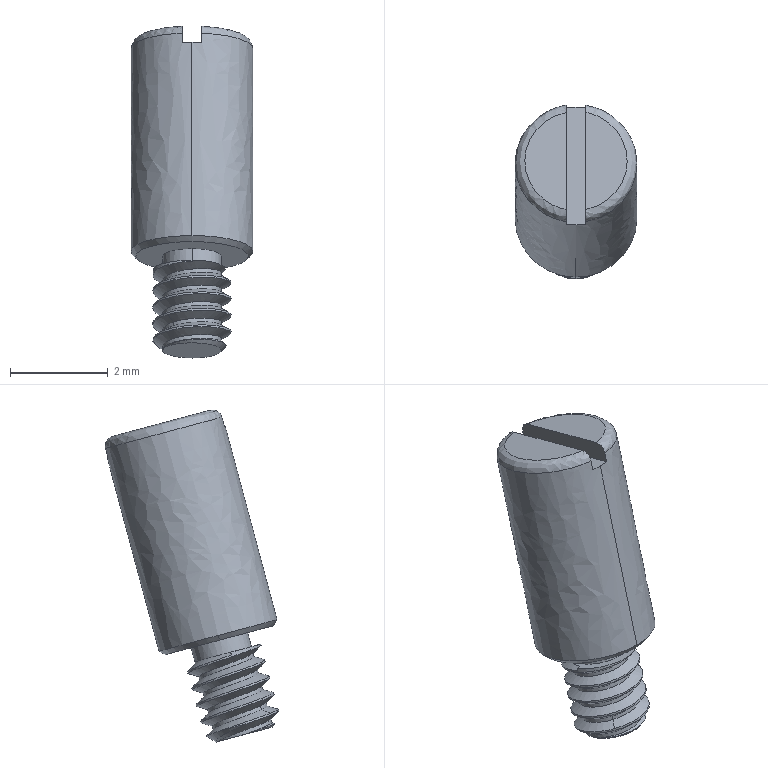Part | SolidWorks | features BaseBody 1 | 1 solid | 33 faces | box 2.5 x 3.555 x 6.804 mm | volume 24.947 mm3 | spline 33